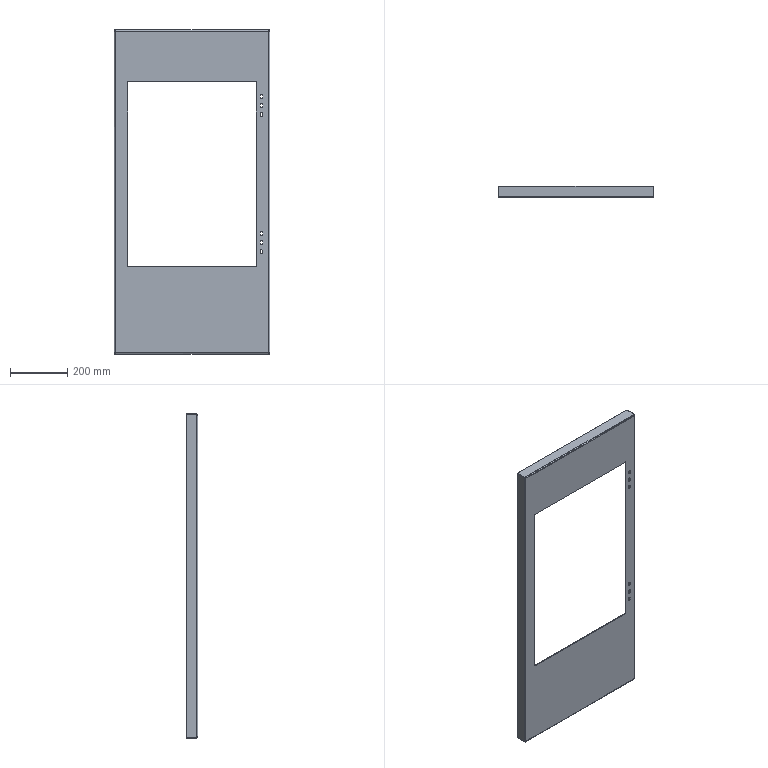Part | SolidWorks | features ICE 2, EdgeFlange 1, FlatPattern 1, SMBaseFlange 1, SheetMetal 1 | 1 solid | 76 faces | box 546 x 40 x 1135 mm | volume 898640 mm3 | plane 38 | cylinder 30 | spline 8 | commonest cylinder face diameters 9 x18 4 x8 8 x4